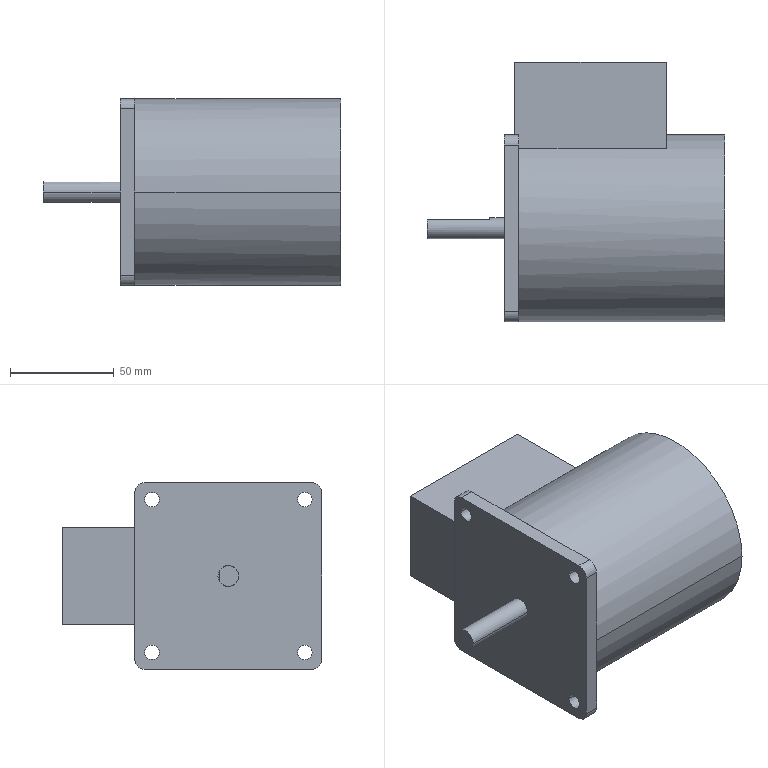Part | STEP file | 40W JSCC motor | 1 solid | 34 faces | box 143 x 125 x 90 mm | volume 815322 mm3 | plane 18 | cylinder 16 | commonest cylinder face diameters 7 x8 10 x6 90 x2